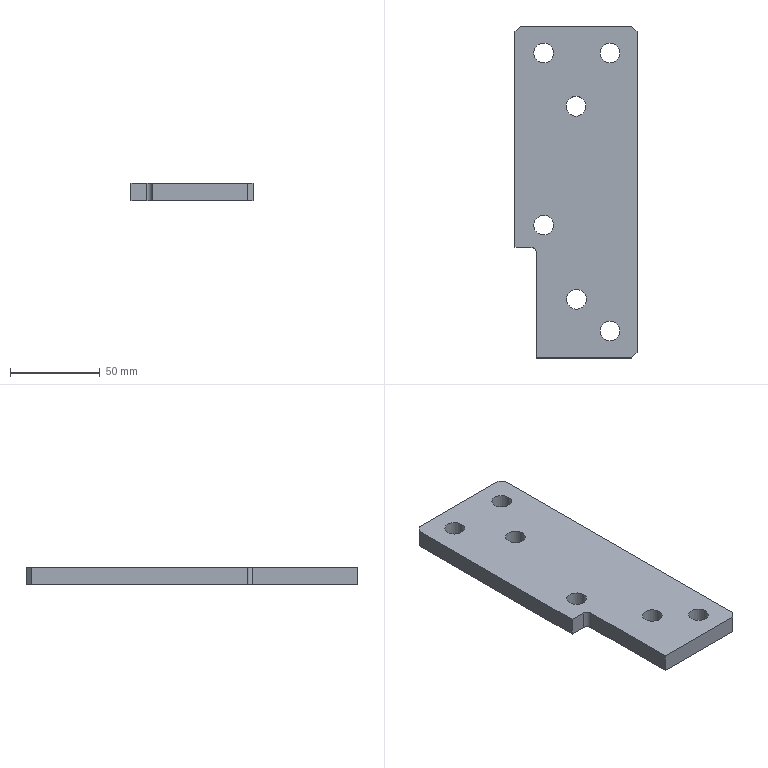Part | STEP file | 1_id182_x_t | 1 solid | 18 faces | box 68 x 185 x 10 mm | volume 112684 mm3 | plane 11 | cylinder 7 | commonest cylinder face diameters 11 x6 6 x1
STEP:
#1=CARTESIAN_POINT('',(0.,0.,0.));
#2=DIRECTION('',(0.,0.,1.));
#3=DIRECTION('',(1.,0.,0.));
#4=AXIS2_PLACEMENT_3D('',#1,#2,#3);
#5=CARTESIAN_POINT('',(251.8,221.703,100.11));
#6=VERTEX_POINT('',#5);
#7=CARTESIAN_POINT('',(246.3,221.703,100.11));
#8=DIRECTION('',(0.,0.,-1.));
#9=DIRECTION('',(1.,0.,0.));
#10=AXIS2_PLACEMENT_3D('',#7,#8,#9);
#11=CIRCLE('',#10,5.5);
#12=CARTESIAN_POINT('',(246.3,221.703,-100.11));
#13=DIRECTION('',(0.,0.,1.));
#14=DIRECTION('',(1.,0.,0.));
#15=AXIS2_PLACEMENT_3D('',#12,#13,#14);
#16=CYLINDRICAL_SURFACE('',#15,5.5);
#17=CARTESIAN_POINT('',(6.283,200.22));
#18=DIRECTION('',(-1.,0.));
#19=VECTOR('',#18,1.);
#20=LINE('',#17,#19);
#21=(GEOMETRIC_REPRESENTATION_CONTEXT(2)PARAMETRIC_REPRESENTATION_CONTEXT()REPRESENTATION_CONTEXT('',''));
#22=DEFINITIONAL_REPRESENTATION('',(#20),#21);
#23=PCURVE('',#16,#22);
#24=CARTESIAN_POINT('',(296.763,161.703,100.11));
#25=DIRECTION('',(0.,0.,1.));
#26=DIRECTION('',(1.,0.,0.));
#27=AXIS2_PLACEMENT_3D('',#24,#25,#26);
#28=PLANE('',#27);
#29=CARTESIAN_POINT('',(-44.962,60.));
#30=CARTESIAN_POINT('',(-44.962,50.474));
#31=CARTESIAN_POINT('',(-53.212,55.237));
#32=CARTESIAN_POINT('',(-61.462,60.));
#33=CARTESIAN_POINT('',(-53.212,64.763));
#34=CARTESIAN_POINT('',(-44.962,69.526));
#35=CARTESIAN_POINT('',(-44.962,60.));
#36=(BOUNDED_CURVE()B_SPLINE_CURVE(2,(#29,#30,#31,#32,#33,#34,#35),.UNSPECIFIED.,.T.,.F.)B_SPLINE_CURVE_WITH_KNOTS((1,2,2,2,2,1),(-2.094,0.,2.094,4.189,6.283,8.378),.UNSPECIFIED.)CURVE()GEOMETRIC_REPRESENTATION_ITEM()RATIONAL_B_SPLINE_CURVE((1.,0.5,1.,0.5,1.,0.5,1.))REPRESENTATION_ITEM(''));
#37=(GEOMETRIC_REPRESENTATION_CONTEXT(2)PARAMETRIC_REPRESENTATION_CONTEXT()REPRESENTATION_CONTEXT('',''));
#38=DEFINITIONAL_REPRESENTATION('',(#36),#37);
#39=PCURVE('',#28,#38);
#40=SURFACE_CURVE('',#11,(#23,#39),.PCURVE_S1.);
#41=EDGE_CURVE('',#6,#6,#40,.T.);
#42=ORIENTED_EDGE('',*,*,#41,.T.);
#43=CARTESIAN_POINT('',(251.8,221.703,90.11));
#44=VERTEX_POINT('',#43);
#45=CARTESIAN_POINT('',(251.8,221.703,90.11));
#46=CARTESIAN_POINT('',(251.8,221.703,100.11));
#47=B_SPLINE_CURVE_WITH_KNOTS('',1,(#45,#46),.UNSPECIFIED.,.F.,.F.,(2,2),(190.22,200.22),.PIECEWISE_BEZIER_KNOTS.);
#48=CARTESIAN_POINT('',(0.,0.));
#49=DIRECTION('',(0.,1.));
#50=VECTOR('',#49,1.);
#51=LINE('',#48,#50);
#52=(GEOMETRIC_REPRESENTATION_CONTEXT(2)PARAMETRIC_REPRESENTATION_CONTEXT()REPRESENTATION_CONTEXT('',''));
#53=DEFINITIONAL_REPRESENTATION('',(#51),#52);
#54=PCURVE('',#16,#53);
#55=CARTESIAN_POINT('',(6.283,0.));
#56=DIRECTION('',(0.,1.));
#57=VECTOR('',#56,1.);
#58=LINE('',#55,#57);
#59=(GEOMETRIC_REPRESENTATION_CONTEXT(2)PARAMETRIC_REPRESENTATION_CONTEXT()REPRESENTATION_CONTEXT('',''));
#60=DEFINITIONAL_REPRESENTATION('',(#58),#59);
#61=PCURVE('',#16,#60);
#62=SEAM_CURVE('',#47,(#54,#61),.PCURVE_S1.);
#63=EDGE_CURVE('',#44,#6,#62,.T.);
#64=ORIENTED_EDGE('',*,*,#63,.F.);
#65=CARTESIAN_POINT('',(246.3,221.703,90.11));
#66=DIRECTION('',(0.,0.,-1.));
#67=DIRECTION('',(1.,0.,0.));
#68=AXIS2_PLACEMENT_3D('',#65,#66,#67);
#69=CIRCLE('',#68,5.5);
#70=CARTESIAN_POINT('',(6.283,190.22));
#71=DIRECTION('',(-1.,0.));
#72=VECTOR('',#71,1.);
#73=LINE('',#70,#72);
#74=(GEOMETRIC_REPRESENTATION_CONTEXT(2)PARAMETRIC_REPRESENTATION_CONTEXT()REPRESENTATION_CONTEXT('',''));
#75=DEFINITIONAL_REPRESENTATION('',(#73),#74);
#76=PCURVE('',#16,#75);
#77=CARTESIAN_POINT('',(296.763,161.703,90.11));
#78=DIRECTION('',(0.,0.,1.));
#79=DIRECTION('',(1.,0.,0.));
#80=AXIS2_PLACEMENT_3D('',#77,#78,#79);
#81=PLANE('',#80);
#82=CARTESIAN_POINT('',(-44.962,60.));
#83=CARTESIAN_POINT('',(-44.962,50.474));
#84=CARTESIAN_POINT('',(-53.212,55.237));
#85=CARTESIAN_POINT('',(-61.462,60.));
#86=CARTESIAN_POINT('',(-53.212,64.763));
#87=CARTESIAN_POINT('',(-44.962,69.526));
#88=CARTESIAN_POINT('',(-44.962,60.));
#89=(BOUNDED_CURVE()B_SPLINE_CURVE(2,(#82,#83,#84,#85,#86,#87,#88),.UNSPECIFIED.,.T.,.F.)B_SPLINE_CURVE_WITH_KNOTS((1,2,2,2,2,1),(-2.094,0.,2.094,4.189,6.283,8.378),.UNSPECIFIED.)CURVE()GEOMETRIC_REPRESENTATION_ITEM()RATIONAL_B_SPLINE_CURVE((1.,0.5,1.,0.5,1.,0.5,1.))REPRESENTATION_ITEM(''));
#90=(GEOMETRIC_REPRESENTATION_CONTEXT(2)PARAMETRIC_REPRESENTATION_CONTEXT()REPRESENTATION_CONTEXT('',''));
#91=DEFINITIONAL_REPRESENTATION('',(#89),#90);
#92=PCURVE('',#81,#91);
#93=SURFACE_CURVE('',#69,(#76,#92),.PCURVE_S1.);
#94=EDGE_CURVE('',#44,#44,#93,.T.);
#95=ORIENTED_EDGE('',*,*,#94,.F.);
#96=ORIENTED_EDGE('',*,*,#63,.T.);
#97=EDGE_LOOP('',(#42,#64,#95,#96));
#98=FACE_BOUND('',#97,.F.);
#99=ADVANCED_FACE('',(#98),#16,.F.);
#100=CARTESIAN_POINT('',(295.3,332.703,90.11));
#101=VERTEX_POINT('',#100);
#102=CARTESIAN_POINT('',(295.3,332.703,100.11));
#103=VERTEX_POINT('',#102);
#104=CARTESIAN_POINT('',(295.3,332.703,90.11));
#105=DIRECTION('',(0.,0.,1.));
#106=VECTOR('',#105,1.);
#107=LINE('',#104,#106);
#108=CARTESIAN_POINT('',(373.531,254.472,100.11));
#109=DIRECTION('',(-0.7071,-0.7071,0.));
#110=DIRECTION('',(0.7071,-0.7071,0.));
#111=AXIS2_PLACEMENT_3D('',#108,#109,#110);
#112=PLANE('',#111);
#113=CARTESIAN_POINT('',(-110.636,-10.));
#114=DIRECTION('',(0.,1.));
#115=VECTOR('',#114,1.);
#116=LINE('',#113,#115);
#117=(GEOMETRIC_REPRESENTATION_CONTEXT(2)PARAMETRIC_REPRESENTATION_CONTEXT()REPRESENTATION_CONTEXT('',''));
#118=DEFINITIONAL_REPRESENTATION('',(#116),#117);
#119=PCURVE('',#112,#118);
#120=CARTESIAN_POINT('',(296.763,332.703,100.11));
#121=DIRECTION('',(0.,-1.,0.));
#122=DIRECTION('',(0.,0.,1.));
#123=AXIS2_PLACEMENT_3D('',#120,#121,#122);
#124=PLANE('',#123);
#125=CARTESIAN_POINT('',(-10.,1.462));
#126=DIRECTION('',(1.,0.));
#127=VECTOR('',#126,1.);
#128=LINE('',#125,#127);
#129=(GEOMETRIC_REPRESENTATION_CONTEXT(2)PARAMETRIC_REPRESENTATION_CONTEXT()REPRESENTATION_CONTEXT('',''));
#130=DEFINITIONAL_REPRESENTATION('',(#128),#129);
#131=PCURVE('',#124,#130);
#132=SURFACE_CURVE('',#107,(#119,#131),.PCURVE_S1.);
#133=EDGE_CURVE('',#101,#103,#132,.T.);
#134=ORIENTED_EDGE('',*,*,#133,.T.);
#135=CARTESIAN_POINT('',(298.3,329.703,100.11));
#136=VERTEX_POINT('',#135);
#137=CARTESIAN_POINT('',(298.3,329.703,100.11));
#138=DIRECTION('',(-0.7071,0.7071,0.));
#139=VECTOR('',#138,1.);
#140=LINE('',#137,#139);
#141=CARTESIAN_POINT('',(-106.393,0.));
#142=DIRECTION('',(-1.,0.));
#143=VECTOR('',#142,1.);
#144=LINE('',#141,#143);
#145=(GEOMETRIC_REPRESENTATION_CONTEXT(2)PARAMETRIC_REPRESENTATION_CONTEXT()REPRESENTATION_CONTEXT('',''));
#146=DEFINITIONAL_REPRESENTATION('',(#144),#145);
#147=PCURVE('',#112,#146);
#148=CARTESIAN_POINT('',(1.538,168.));
#149=DIRECTION('',(-0.7071,0.7071));
#150=VECTOR('',#149,1.);
#151=LINE('',#148,#150);
#152=(GEOMETRIC_REPRESENTATION_CONTEXT(2)PARAMETRIC_REPRESENTATION_CONTEXT()REPRESENTATION_CONTEXT('',''));
#153=DEFINITIONAL_REPRESENTATION('',(#151),#152);
#154=PCURVE('',#28,#153);
#155=SURFACE_CURVE('',#140,(#147,#154),.PCURVE_S1.);
#156=EDGE_CURVE('',#136,#103,#155,.T.);
#157=ORIENTED_EDGE('',*,*,#156,.F.);
#158=CARTESIAN_POINT('',(298.3,329.703,90.11));
#159=VERTEX_POINT('',#158);
#160=CARTESIAN_POINT('',(298.3,329.703,90.11));
#161=DIRECTION('',(0.,0.,1.));
#162=VECTOR('',#161,1.);
#163=LINE('',#160,#162);
#164=CARTESIAN_POINT('',(-106.393,-10.));
#165=DIRECTION('',(0.,1.));
#166=VECTOR('',#165,1.);
#167=LINE('',#164,#166);
#168=(GEOMETRIC_REPRESENTATION_CONTEXT(2)PARAMETRIC_REPRESENTATION_CONTEXT()REPRESENTATION_CONTEXT('',''));
#169=DEFINITIONAL_REPRESENTATION('',(#167),#168);
#170=PCURVE('',#112,#169);
#171=CARTESIAN_POINT('',(298.3,316.703,100.11));
#172=DIRECTION('',(-1.,0.,0.));
#173=DIRECTION('',(0.,-1.,0.));
#174=AXIS2_PLACEMENT_3D('',#171,#172,#173);
#175=PLANE('',#174);
#176=CARTESIAN_POINT('',(-13.,-10.));
#177=DIRECTION('',(0.,1.));
#178=VECTOR('',#177,1.);
#179=LINE('',#176,#178);
#180=(GEOMETRIC_REPRESENTATION_CONTEXT(2)PARAMETRIC_REPRESENTATION_CONTEXT()REPRESENTATION_CONTEXT('',''));
#181=DEFINITIONAL_REPRESENTATION('',(#179),#180);
#182=PCURVE('',#175,#181);
#183=SURFACE_CURVE('',#163,(#170,#182),.PCURVE_S1.);
#184=EDGE_CURVE('',#159,#136,#183,.T.);
#185=ORIENTED_EDGE('',*,*,#184,.F.);
#186=CARTESIAN_POINT('',(295.3,332.703,90.11));
#187=DIRECTION('',(0.7071,-0.7071,0.));
#188=VECTOR('',#187,1.);
#189=LINE('',#186,#188);
#190=CARTESIAN_POINT('',(-110.636,-10.));
#191=DIRECTION('',(1.,0.));
#192=VECTOR('',#191,1.);
#193=LINE('',#190,#192);
#194=(GEOMETRIC_REPRESENTATION_CONTEXT(2)PARAMETRIC_REPRESENTATION_CONTEXT()REPRESENTATION_CONTEXT('',''));
#195=DEFINITIONAL_REPRESENTATION('',(#193),#194);
#196=PCURVE('',#112,#195);
#197=CARTESIAN_POINT('',(-1.462,171.));
#198=DIRECTION('',(0.7071,-0.7071));
#199=VECTOR('',#198,1.);
#200=LINE('',#197,#199);
#201=(GEOMETRIC_REPRESENTATION_CONTEXT(2)PARAMETRIC_REPRESENTATION_CONTEXT()REPRESENTATION_CONTEXT('',''));
#202=DEFINITIONAL_REPRESENTATION('',(#200),#201);
#203=PCURVE('',#81,#202);
#204=SURFACE_CURVE('',#189,(#196,#203),.PCURVE_S1.);
#205=EDGE_CURVE('',#101,#159,#204,.T.);
#206=ORIENTED_EDGE('',*,*,#205,.F.);
#207=EDGE_LOOP('',(#134,#157,#185,#206));
#208=FACE_BOUND('',#207,.T.);
#209=ADVANCED_FACE('',(#208),#112,.F.);
#210=CARTESIAN_POINT('',(233.3,332.703,90.11));
#211=VERTEX_POINT('',#210);
#212=CARTESIAN_POINT('',(233.3,332.703,100.11));
#213=VERTEX_POINT('',#212);
#214=CARTESIAN_POINT('',(233.3,332.703,90.11));
#215=DIRECTION('',(0.,0.,1.));
#216=VECTOR('',#215,1.);
#217=LINE('',#214,#216);
#218=CARTESIAN_POINT('',(-10.,63.462));
#219=DIRECTION('',(1.,0.));
#220=VECTOR('',#219,1.);
#221=LINE('',#218,#220);
#222=(GEOMETRIC_REPRESENTATION_CONTEXT(2)PARAMETRIC_REPRESENTATION_CONTEXT()REPRESENTATION_CONTEXT('',''));
#223=DEFINITIONAL_REPRESENTATION('',(#221),#222);
#224=PCURVE('',#124,#223);
#225=CARTESIAN_POINT('',(187.531,286.935,100.11));
#226=DIRECTION('',(0.7071,-0.7071,0.));
#227=DIRECTION('',(0.7071,0.7071,0.));
#228=AXIS2_PLACEMENT_3D('',#225,#226,#227);
#229=PLANE('',#228);
#230=CARTESIAN_POINT('',(64.727,-10.));
#231=DIRECTION('',(0.,1.));
#232=VECTOR('',#231,1.);
#233=LINE('',#230,#232);
#234=(GEOMETRIC_REPRESENTATION_CONTEXT(2)PARAMETRIC_REPRESENTATION_CONTEXT()REPRESENTATION_CONTEXT('',''));
#235=DEFINITIONAL_REPRESENTATION('',(#233),#234);
#236=PCURVE('',#229,#235);
#237=SURFACE_CURVE('',#217,(#224,#236),.PCURVE_S1.);
#238=EDGE_CURVE('',#211,#213,#237,.T.);
#239=ORIENTED_EDGE('',*,*,#238,.T.);
#240=CARTESIAN_POINT('',(233.3,332.703,100.11));
#241=DIRECTION('',(1.,0.,0.));
#242=VECTOR('',#241,1.);
#243=LINE('',#240,#242);
#244=CARTESIAN_POINT('',(0.,63.462));
#245=DIRECTION('',(0.,-1.));
#246=VECTOR('',#245,1.);
#247=LINE('',#244,#246);
#248=(GEOMETRIC_REPRESENTATION_CONTEXT(2)PARAMETRIC_REPRESENTATION_CONTEXT()REPRESENTATION_CONTEXT('',''));
#249=DEFINITIONAL_REPRESENTATION('',(#247),#248);
#250=PCURVE('',#124,#249);
#251=CARTESIAN_POINT('',(-63.462,171.));
#252=DIRECTION('',(1.,0.));
#253=VECTOR('',#252,1.);
#254=LINE('',#251,#253);
#255=(GEOMETRIC_REPRESENTATION_CONTEXT(2)PARAMETRIC_REPRESENTATION_CONTEXT()REPRESENTATION_CONTEXT('',''));
#256=DEFINITIONAL_REPRESENTATION('',(#254),#255);
#257=PCURVE('',#28,#256);
#258=SURFACE_CURVE('',#243,(#250,#257),.PCURVE_S1.);
#259=EDGE_CURVE('',#213,#103,#258,.T.);
#260=ORIENTED_EDGE('',*,*,#259,.T.);
#261=ORIENTED_EDGE('',*,*,#133,.F.);
#262=CARTESIAN_POINT('',(233.3,332.703,90.11));
#263=DIRECTION('',(1.,0.,0.));
#264=VECTOR('',#263,1.);
#265=LINE('',#262,#264);
#266=CARTESIAN_POINT('',(-10.,63.462));
#267=DIRECTION('',(0.,-1.));
#268=VECTOR('',#267,1.);
#269=LINE('',#266,#268);
#270=(GEOMETRIC_REPRESENTATION_CONTEXT(2)PARAMETRIC_REPRESENTATION_CONTEXT()REPRESENTATION_CONTEXT('',''));
#271=DEFINITIONAL_REPRESENTATION('',(#269),#270);
#272=PCURVE('',#124,#271);
#273=CARTESIAN_POINT('',(-63.462,171.));
#274=DIRECTION('',(1.,0.));
#275=VECTOR('',#274,1.);
#276=LINE('',#273,#275);
#277=(GEOMETRIC_REPRESENTATION_CONTEXT(2)PARAMETRIC_REPRESENTATION_CONTEXT()REPRESENTATION_CONTEXT('',''));
#278=DEFINITIONAL_REPRESENTATION('',(#276),#277);
#279=PCURVE('',#81,#278);
#280=SURFACE_CURVE('',#265,(#272,#279),.PCURVE_S1.);
#281=EDGE_CURVE('',#211,#101,#280,.T.);
#282=ORIENTED_EDGE('',*,*,#281,.F.);
#283=EDGE_LOOP('',(#239,#260,#261,#282));
#284=FACE_BOUND('',#283,.T.);
#285=ADVANCED_FACE('',(#284),#124,.F.);
#286=CARTESIAN_POINT('',(230.3,329.703,90.11));
#287=VERTEX_POINT('',#286);
#288=CARTESIAN_POINT('',(230.3,329.703,100.11));
#289=VERTEX_POINT('',#288);
#290=CARTESIAN_POINT('',(230.3,329.703,90.11));
#291=DIRECTION('',(0.,0.,1.));
#292=VECTOR('',#291,1.);
#293=LINE('',#290,#292);
#294=CARTESIAN_POINT('',(60.484,-10.));
#295=DIRECTION('',(0.,1.));
#296=VECTOR('',#295,1.);
#297=LINE('',#294,#296);
#298=(GEOMETRIC_REPRESENTATION_CONTEXT(2)PARAMETRIC_REPRESENTATION_CONTEXT()REPRESENTATION_CONTEXT('',''));
#299=DEFINITIONAL_REPRESENTATION('',(#297),#298);
#300=PCURVE('',#229,#299);
#301=CARTESIAN_POINT('',(230.3,316.703,100.11));
#302=DIRECTION('',(1.,0.,0.));
#303=DIRECTION('',(0.,1.,0.));
#304=AXIS2_PLACEMENT_3D('',#301,#302,#303);
#305=PLANE('',#304);
#306=CARTESIAN_POINT('',(13.,-10.));
#307=DIRECTION('',(0.,1.));
#308=VECTOR('',#307,1.);
#309=LINE('',#306,#308);
#310=(GEOMETRIC_REPRESENTATION_CONTEXT(2)PARAMETRIC_REPRESENTATION_CONTEXT()REPRESENTATION_CONTEXT('',''));
#311=DEFINITIONAL_REPRESENTATION('',(#309),#310);
#312=PCURVE('',#305,#311);
#313=SURFACE_CURVE('',#293,(#300,#312),.PCURVE_S1.);
#314=EDGE_CURVE('',#287,#289,#313,.T.);
#315=ORIENTED_EDGE('',*,*,#314,.T.);
#316=CARTESIAN_POINT('',(233.3,332.703,100.11));
#317=DIRECTION('',(-0.7071,-0.7071,0.));
#318=VECTOR('',#317,1.);
#319=LINE('',#316,#318);
#320=CARTESIAN_POINT('',(64.727,0.));
#321=DIRECTION('',(-1.,0.));
#322=VECTOR('',#321,1.);
#323=LINE('',#320,#322);
#324=(GEOMETRIC_REPRESENTATION_CONTEXT(2)PARAMETRIC_REPRESENTATION_CONTEXT()REPRESENTATION_CONTEXT('',''));
#325=DEFINITIONAL_REPRESENTATION('',(#323),#324);
#326=PCURVE('',#229,#325);
#327=CARTESIAN_POINT('',(-63.462,171.));
#328=DIRECTION('',(-0.7071,-0.7071));
#329=VECTOR('',#328,1.);
#330=LINE('',#327,#329);
#331=(GEOMETRIC_REPRESENTATION_CONTEXT(2)PARAMETRIC_REPRESENTATION_CONTEXT()REPRESENTATION_CONTEXT('',''));
#332=DEFINITIONAL_REPRESENTATION('',(#330),#331);
#333=PCURVE('',#28,#332);
#334=SURFACE_CURVE('',#319,(#326,#333),.PCURVE_S1.);
#335=EDGE_CURVE('',#213,#289,#334,.T.);
#336=ORIENTED_EDGE('',*,*,#335,.F.);
#337=ORIENTED_EDGE('',*,*,#238,.F.);
#338=CARTESIAN_POINT('',(230.3,329.703,90.11));
#339=DIRECTION('',(0.7071,0.7071,0.));
#340=VECTOR('',#339,1.);
#341=LINE('',#338,#340);
#342=CARTESIAN_POINT('',(60.484,-10.));
#343=DIRECTION('',(1.,0.));
#344=VECTOR('',#343,1.);
#345=LINE('',#342,#344);
#346=(GEOMETRIC_REPRESENTATION_CONTEXT(2)PARAMETRIC_REPRESENTATION_CONTEXT()REPRESENTATION_CONTEXT('',''));
#347=DEFINITIONAL_REPRESENTATION('',(#345),#346);
#348=PCURVE('',#229,#347);
#349=CARTESIAN_POINT('',(-66.463,168.));
#350=DIRECTION('',(0.7071,0.7071));
#351=VECTOR('',#350,1.);
#352=LINE('',#349,#351);
#353=(GEOMETRIC_REPRESENTATION_CONTEXT(2)PARAMETRIC_REPRESENTATION_CONTEXT()REPRESENTATION_CONTEXT('',''));
#354=DEFINITIONAL_REPRESENTATION('',(#352),#353);
#355=PCURVE('',#81,#354);
#356=SURFACE_CURVE('',#341,(#348,#355),.PCURVE_S1.);
#357=EDGE_CURVE('',#287,#211,#356,.T.);
#358=ORIENTED_EDGE('',*,*,#357,.F.);
#359=EDGE_LOOP('',(#315,#336,#337,#358));
#360=FACE_BOUND('',#359,.T.);
#361=ADVANCED_FACE('',(#360),#229,.F.);
#362=CARTESIAN_POINT('',(230.3,209.297,100.11));
#363=VERTEX_POINT('',#362);
#364=CARTESIAN_POINT('',(230.3,209.297,100.11));
#365=DIRECTION('',(0.,1.,0.));
#366=VECTOR('',#365,1.);
#367=LINE('',#364,#366);
#368=CARTESIAN_POINT('',(-107.407,0.));
#369=DIRECTION('',(1.,0.));
#370=VECTOR('',#369,1.);
#371=LINE('',#368,#370);
#372=(GEOMETRIC_REPRESENTATION_CONTEXT(2)PARAMETRIC_REPRESENTATION_CONTEXT()REPRESENTATION_CONTEXT('',''));
#373=DEFINITIONAL_REPRESENTATION('',(#371),#372);
#374=PCURVE('',#305,#373);
#375=CARTESIAN_POINT('',(-66.463,47.593));
#376=DIRECTION('',(0.,1.));
#377=VECTOR('',#376,1.);
#378=LINE('',#375,#377);
#379=(GEOMETRIC_REPRESENTATION_CONTEXT(2)PARAMETRIC_REPRESENTATION_CONTEXT()REPRESENTATION_CONTEXT('',''));
#380=DEFINITIONAL_REPRESENTATION('',(#378),#379);
#381=PCURVE('',#28,#380);
#382=SURFACE_CURVE('',#367,(#374,#381),.PCURVE_S1.);
#383=EDGE_CURVE('',#363,#289,#382,.T.);
#384=ORIENTED_EDGE('',*,*,#383,.T.);
#385=ORIENTED_EDGE('',*,*,#314,.F.);
#386=CARTESIAN_POINT('',(230.3,209.297,90.11));
#387=VERTEX_POINT('',#386);
#388=CARTESIAN_POINT('',(230.3,209.297,90.11));
#389=DIRECTION('',(0.,1.,0.));
#390=VECTOR('',#389,1.);
#391=LINE('',#388,#390);
#392=CARTESIAN_POINT('',(-107.407,-10.));
#393=DIRECTION('',(1.,0.));
#394=VECTOR('',#393,1.);
#395=LINE('',#392,#394);
#396=(GEOMETRIC_REPRESENTATION_CONTEXT(2)PARAMETRIC_REPRESENTATION_CONTEXT()REPRESENTATION_CONTEXT('',''));
#397=DEFINITIONAL_REPRESENTATION('',(#395),#396);
#398=PCURVE('',#305,#397);
#399=CARTESIAN_POINT('',(-66.463,47.593));
#400=DIRECTION('',(0.,1.));
#401=VECTOR('',#400,1.);
#402=LINE('',#399,#401);
#403=(GEOMETRIC_REPRESENTATION_CONTEXT(2)PARAMETRIC_REPRESENTATION_CONTEXT()REPRESENTATION_CONTEXT('',''));
#404=DEFINITIONAL_REPRESENTATION('',(#402),#403);
#405=PCURVE('',#81,#404);
#406=SURFACE_CURVE('',#391,(#398,#405),.PCURVE_S1.);
#407=EDGE_CURVE('',#387,#287,#406,.T.);
#408=ORIENTED_EDGE('',*,*,#407,.F.);
#409=CARTESIAN_POINT('',(230.3,209.297,90.11));
#410=DIRECTION('',(0.,0.,1.));
#411=VECTOR('',#410,1.);
#412=LINE('',#409,#411);
#413=CARTESIAN_POINT('',(-107.407,-10.));
#414=DIRECTION('',(0.,1.));
#415=VECTOR('',#414,1.);
#416=LINE('',#413,#415);
#417=(GEOMETRIC_REPRESENTATION_CONTEXT(2)PARAMETRIC_REPRESENTATION_CONTEXT()REPRESENTATION_CONTEXT('',''));
#418=DEFINITIONAL_REPRESENTATION('',(#416),#417);
#419=PCURVE('',#305,#418);
#420=CARTESIAN_POINT('',(174.688,209.297,100.11));
#421=DIRECTION('',(0.,-1.,0.));
#422=DIRECTION('',(0.,0.,-1.));
#423=AXIS2_PLACEMENT_3D('',#420,#421,#422);
#424=PLANE('',#423);
#425=CARTESIAN_POINT('',(10.,55.612));
#426=DIRECTION('',(-1.,0.));
#427=VECTOR('',#426,1.);
#428=LINE('',#425,#427);
#429=(GEOMETRIC_REPRESENTATION_CONTEXT(2)PARAMETRIC_REPRESENTATION_CONTEXT()REPRESENTATION_CONTEXT('',''));
#430=DEFINITIONAL_REPRESENTATION('',(#428),#429);
#431=PCURVE('',#424,#430);
#432=SURFACE_CURVE('',#412,(#419,#431),.PCURVE_S1.);
#433=EDGE_CURVE('',#387,#363,#432,.T.);
#434=ORIENTED_EDGE('',*,*,#433,.T.);
#435=EDGE_LOOP('',(#384,#385,#408,#434));
#436=FACE_BOUND('',#435,.T.);
#437=ADVANCED_FACE('',(#436),#305,.F.);
#438=CARTESIAN_POINT('',(239.15,209.297,100.11));
#439=VERTEX_POINT('',#438);
#440=CARTESIAN_POINT('',(239.15,209.297,90.11));
#441=VERTEX_POINT('',#440);
#442=CARTESIAN_POINT('',(239.15,209.297,100.11));
#443=DIRECTION('',(0.,0.,-1.));
#444=VECTOR('',#443,1.);
#445=LINE('',#442,#444);
#446=CARTESIAN_POINT('',(0.,64.463));
#447=DIRECTION('',(1.,0.));
#448=VECTOR('',#447,1.);
#449=LINE('',#446,#448);
#450=(GEOMETRIC_REPRESENTATION_CONTEXT(2)PARAMETRIC_REPRESENTATION_CONTEXT()REPRESENTATION_CONTEXT('',''));
#451=DEFINITIONAL_REPRESENTATION('',(#449),#450);
#452=PCURVE('',#424,#451);
#453=CARTESIAN_POINT('',(239.15,206.297,100.11));
#454=DIRECTION('',(0.,0.,-1.));
#455=DIRECTION('',(-1.,0.,0.));
#456=AXIS2_PLACEMENT_3D('',#453,#454,#455);
#457=CYLINDRICAL_SURFACE('',#456,3.);
#458=CARTESIAN_POINT('',(1.571,0.));
#459=DIRECTION('',(0.,1.));
#460=VECTOR('',#459,1.);
#461=LINE('',#458,#460);
#462=(GEOMETRIC_REPRESENTATION_CONTEXT(2)PARAMETRIC_REPRESENTATION_CONTEXT()REPRESENTATION_CONTEXT('',''));
#463=DEFINITIONAL_REPRESENTATION('',(#461),#462);
#464=PCURVE('',#457,#463);
#465=SURFACE_CURVE('',#445,(#452,#464),.PCURVE_S1.);
#466=EDGE_CURVE('',#439,#441,#465,.T.);
#467=ORIENTED_EDGE('',*,*,#466,.F.);
#468=CARTESIAN_POINT('',(239.15,209.297,100.11));
#469=DIRECTION('',(-1.,0.,0.));
#470=VECTOR('',#469,1.);
#471=LINE('',#468,#470);
#472=CARTESIAN_POINT('',(0.,64.463));
#473=DIRECTION('',(0.,-1.));
#474=VECTOR('',#473,1.);
#475=LINE('',#472,#474);
#476=(GEOMETRIC_REPRESENTATION_CONTEXT(2)PARAMETRIC_REPRESENTATION_CONTEXT()REPRESENTATION_CONTEXT('',''));
#477=DEFINITIONAL_REPRESENTATION('',(#475),#476);
#478=PCURVE('',#424,#477);
#479=CARTESIAN_POINT('',(-57.612,47.593));
#480=DIRECTION('',(-1.,0.));
#481=VECTOR('',#480,1.);
#482=LINE('',#479,#481);
#483=(GEOMETRIC_REPRESENTATION_CONTEXT(2)PARAMETRIC_REPRESENTATION_CONTEXT()REPRESENTATION_CONTEXT('',''));
#484=DEFINITIONAL_REPRESENTATION('',(#482),#483);
#485=PCURVE('',#28,#484);
#486=SURFACE_CURVE('',#471,(#478,#485),.PCURVE_S1.);
#487=EDGE_CURVE('',#439,#363,#486,.T.);
#488=ORIENTED_EDGE('',*,*,#487,.T.);
#489=ORIENTED_EDGE('',*,*,#433,.F.);
#490=CARTESIAN_POINT('',(239.15,209.297,90.11));
#491=DIRECTION('',(-1.,0.,0.));
#492=VECTOR('',#491,1.);
#493=LINE('',#490,#492);
#494=CARTESIAN_POINT('',(10.,64.463));
#495=DIRECTION('',(0.,-1.));
#496=VECTOR('',#495,1.);
#497=LINE('',#494,#496);
#498=(GEOMETRIC_REPRESENTATION_CONTEXT(2)PARAMETRIC_REPRESENTATION_CONTEXT()REPRESENTATION_CONTEXT('',''));
#499=DEFINITIONAL_REPRESENTATION('',(#497),#498);
#500=PCURVE('',#424,#499);
#501=CARTESIAN_POINT('',(-57.612,47.593));
#502=DIRECTION('',(-1.,0.));
#503=VECTOR('',#502,1.);
#504=LINE('',#501,#503);
#505=(GEOMETRIC_REPRESENTATION_CONTEXT(2)PARAMETRIC_REPRESENTATION_CONTEXT()REPRESENTATION_CONTEXT('',''));
#506=DEFINITIONAL_REPRESENTATION('',(#504),#505);
#507=PCURVE('',#81,#506);
#508=SURFACE_CURVE('',#493,(#500,#507),.PCURVE_S1.);
#509=EDGE_CURVE('',#441,#387,#508,.T.);
#510=ORIENTED_EDGE('',*,*,#509,.F.);
#511=EDGE_LOOP('',(#467,#488,#489,#510));
#512=FACE_BOUND('',#511,.T.);
#513=ADVANCED_FACE('',(#512),#424,.T.);
#514=CARTESIAN_POINT('',(242.15,206.297,90.11));
#515=VERTEX_POINT('',#514);
#516=CARTESIAN_POINT('',(239.15,206.297,90.11));
#517=DIRECTION('',(0.,0.,1.));
#518=DIRECTION('',(1.,0.,0.));
#519=AXIS2_PLACEMENT_3D('',#516,#517,#518);
#520=CIRCLE('',#519,3.);
#521=CARTESIAN_POINT('',(3.142,10.));
#522=DIRECTION('',(-1.,0.));
#523=VECTOR('',#522,1.);
#524=LINE('',#521,#523);
#525=(GEOMETRIC_REPRESENTATION_CONTEXT(2)PARAMETRIC_REPRESENTATION_CONTEXT()REPRESENTATION_CONTEXT('',''));
#526=DEFINITIONAL_REPRESENTATION('',(#524),#525);
#527=PCURVE('',#457,#526);
#528=CARTESIAN_POINT('',(-57.612,44.593));
#529=DIRECTION('',(1.,0.));
#530=AXIS2_PLACEMENT_2D('',#528,#529);
#531=CIRCLE('',#530,3.);
#532=(GEOMETRIC_REPRESENTATION_CONTEXT(2)PARAMETRIC_REPRESENTATION_CONTEXT()REPRESENTATION_CONTEXT('',''));
#533=DEFINITIONAL_REPRESENTATION('',(#531),#532);
#534=PCURVE('',#81,#533);
#535=SURFACE_CURVE('',#520,(#527,#534),.PCURVE_S1.);
#536=EDGE_CURVE('',#515,#441,#535,.T.);
#537=ORIENTED_EDGE('',*,*,#536,.T.);
#538=ORIENTED_EDGE('',*,*,#466,.F.);
#539=CARTESIAN_POINT('',(242.15,206.297,100.11));
#540=VERTEX_POINT('',#539);
#541=CARTESIAN_POINT('',(239.15,206.297,100.11));
#542=DIRECTION('',(0.,0.,-1.));
#543=DIRECTION('',(0.,1.,0.));
#544=AXIS2_PLACEMENT_3D('',#541,#542,#543);
#545=CIRCLE('',#544,3.);
#546=CARTESIAN_POINT('',(1.571,0.));
#547=DIRECTION('',(1.,0.));
#548=VECTOR('',#547,1.);
#549=LINE('',#546,#548);
#550=(GEOMETRIC_REPRESENTATION_CONTEXT(2)PARAMETRIC_REPRESENTATION_CONTEXT()REPRESENTATION_CONTEXT('',''));
#551=DEFINITIONAL_REPRESENTATION('',(#549),#550);
#552=PCURVE('',#457,#551);
#553=CARTESIAN_POINT('',(-57.612,47.593));
#554=CARTESIAN_POINT('',(-52.416,47.593));
#555=CARTESIAN_POINT('',(-55.014,43.093));
#556=CARTESIAN_POINT('',(-57.612,38.593));
#557=CARTESIAN_POINT('',(-60.211,43.093));
#558=CARTESIAN_POINT('',(-62.809,47.593));
#559=CARTESIAN_POINT('',(-57.612,47.593));
#560=(BOUNDED_CURVE()B_SPLINE_CURVE(2,(#553,#554,#555,#556,#557,#558,#559),.UNSPECIFIED.,.T.,.F.)B_SPLINE_CURVE_WITH_KNOTS((1,2,2,2,2,1),(-2.094,0.,2.094,4.189,6.283,8.378),.UNSPECIFIED.)CURVE()GEOMETRIC_REPRESENTATION_ITEM()RATIONAL_B_SPLINE_CURVE((1.,0.5,1.,0.5,1.,0.5,1.))REPRESENTATION_ITEM(''));
#561=(GEOMETRIC_REPRESENTATION_CONTEXT(2)PARAMETRIC_REPRESENTATION_CONTEXT()REPRESENTATION_CONTEXT('',''));
#562=DEFINITIONAL_REPRESENTATION('',(#560),#561);
#563=PCURVE('',#28,#562);
#564=SURFACE_CURVE('',#545,(#552,#563),.PCURVE_S1.);
#565=EDGE_CURVE('',#439,#540,#564,.T.);
#566=ORIENTED_EDGE('',*,*,#565,.T.);
#567=CARTESIAN_POINT('',(242.15,206.297,90.11));
#568=DIRECTION('',(0.,0.,1.));
#569=VECTOR('',#568,1.);
#570=LINE('',#567,#569);
#571=CARTESIAN_POINT('',(3.142,10.));
#572=DIRECTION('',(0.,-1.));
#573=VECTOR('',#572,1.);
#574=LINE('',#571,#573);
#575=(GEOMETRIC_REPRESENTATION_CONTEXT(2)PARAMETRIC_REPRESENTATION_CONTEXT()REPRESENTATION_CONTEXT('',''));
#576=DEFINITIONAL_REPRESENTATION('',(#574),#575);
#577=PCURVE('',#457,#576);
#578=CARTESIAN_POINT('',(242.15,38.297,100.11));
#579=DIRECTION('',(-1.,0.,0.));
#580=DIRECTION('',(0.,1.,0.));
#581=AXIS2_PLACEMENT_3D('',#578,#579,#580);
#582=PLANE('',#581);
#583=CARTESIAN_POINT('',(168.,10.));
#584=DIRECTION('',(0.,-1.));
#585=VECTOR('',#584,1.);
#586=LINE('',#583,#585);
#587=(GEOMETRIC_REPRESENTATION_CONTEXT(2)PARAMETRIC_REPRESENTATION_CONTEXT()REPRESENTATION_CONTEXT('',''));
#588=DEFINITIONAL_REPRESENTATION('',(#586),#587);
#589=PCURVE('',#582,#588);
#590=SURFACE_CURVE('',#570,(#577,#589),.PCURVE_S1.);
#591=EDGE_CURVE('',#515,#540,#590,.T.);
#592=ORIENTED_EDGE('',*,*,#591,.F.);
#593=EDGE_LOOP('',(#537,#538,#566,#592));
#594=FACE_BOUND('',#593,.F.);
#595=ADVANCED_FACE('',(#594),#457,.F.);
#596=ORIENTED_EDGE('',*,*,#591,.F.);
#597=CARTESIAN_POINT('',(242.15,147.703,90.11));
#598=VERTEX_POINT('',#597);
#599=CARTESIAN_POINT('',(242.15,147.703,90.11));
#600=DIRECTION('',(0.,1.,0.));
#601=VECTOR('',#600,1.);
#602=LINE('',#599,#601);
#603=CARTESIAN_POINT('',(109.407,10.));
#604=DIRECTION('',(1.,0.));
#605=VECTOR('',#604,1.);
#606=LINE('',#603,#605);
#607=(GEOMETRIC_REPRESENTATION_CONTEXT(2)PARAMETRIC_REPRESENTATION_CONTEXT()REPRESENTATION_CONTEXT('',''));
#608=DEFINITIONAL_REPRESENTATION('',(#606),#607);
#609=PCURVE('',#582,#608);
#610=CARTESIAN_POINT('',(-54.612,-14.));
#611=DIRECTION('',(0.,1.));
#612=VECTOR('',#611,1.);
#613=LINE('',#610,#612);
#614=(GEOMETRIC_REPRESENTATION_CONTEXT(2)PARAMETRIC_REPRESENTATION_CONTEXT()REPRESENTATION_CONTEXT('',''));
#615=DEFINITIONAL_REPRESENTATION('',(#613),#614);
#616=PCURVE('',#81,#615);
#617=SURFACE_CURVE('',#602,(#609,#616),.PCURVE_S1.);
#618=EDGE_CURVE('',#598,#515,#617,.T.);
#619=ORIENTED_EDGE('',*,*,#618,.F.);
#620=CARTESIAN_POINT('',(242.15,147.703,100.11));
#621=VERTEX_POINT('',#620);
#622=CARTESIAN_POINT('',(242.15,147.703,100.11));
#623=DIRECTION('',(0.,0.,-1.));
#624=VECTOR('',#623,1.);
#625=LINE('',#622,#624);
#626=CARTESIAN_POINT('',(109.407,0.));
#627=DIRECTION('',(0.,1.));
#628=VECTOR('',#627,1.);
#629=LINE('',#626,#628);
#630=(GEOMETRIC_REPRESENTATION_CONTEXT(2)PARAMETRIC_REPRESENTATION_CONTEXT()REPRESENTATION_CONTEXT('',''));
#631=DEFINITIONAL_REPRESENTATION('',(#629),#630);
#632=PCURVE('',#582,#631);
#633=CARTESIAN_POINT('',(231.838,147.703,100.11));
#634=DIRECTION('',(0.,1.,0.));
#635=DIRECTION('',(0.,0.,-1.));
#636=AXIS2_PLACEMENT_3D('',#633,#634,#635);
#637=PLANE('',#636);
#638=CARTESIAN_POINT('',(0.,-10.312));
#639=DIRECTION('',(1.,0.));
#640=VECTOR('',#639,1.);
#641=LINE('',#638,#640);
#642=(GEOMETRIC_REPRESENTATION_CONTEXT(2)PARAMETRIC_REPRESENTATION_CONTEXT()REPRESENTATION_CONTEXT('',''));
#643=DEFINITIONAL_REPRESENTATION('',(#641),#642);
#644=PCURVE('',#637,#643);
#645=SURFACE_CURVE('',#625,(#632,#644),.PCURVE_S1.);
#646=EDGE_CURVE('',#621,#598,#645,.T.);
#647=ORIENTED_EDGE('',*,*,#646,.F.);
#648=CARTESIAN_POINT('',(242.15,147.703,100.11));
#649=DIRECTION('',(0.,1.,0.));
#650=VECTOR('',#649,1.);
#651=LINE('',#648,#650);
#652=CARTESIAN_POINT('',(109.407,0.));
#653=DIRECTION('',(1.,0.));
#654=VECTOR('',#653,1.);
#655=LINE('',#652,#654);
#656=(GEOMETRIC_REPRESENTATION_CONTEXT(2)PARAMETRIC_REPRESENTATION_CONTEXT()REPRESENTATION_CONTEXT('',''));
#657=DEFINITIONAL_REPRESENTATION('',(#655),#656);
#658=PCURVE('',#582,#657);
#659=CARTESIAN_POINT('',(-54.612,-14.));
#660=DIRECTION('',(0.,1.));
#661=VECTOR('',#660,1.);
#662=LINE('',#659,#661);
#663=(GEOMETRIC_REPRESENTATION_CONTEXT(2)PARAMETRIC_REPRESENTATION_CONTEXT()REPRESENTATION_CONTEXT('',''));
#664=DEFINITIONAL_REPRESENTATION('',(#662),#663);
#665=PCURVE('',#28,#664);
#666=SURFACE_CURVE('',#651,(#658,#665),.PCURVE_S1.);
#667=EDGE_CURVE('',#621,#540,#666,.T.);
#668=ORIENTED_EDGE('',*,*,#667,.T.);
#669=EDGE_LOOP('',(#596,#619,#647,#668));
#670=FACE_BOUND('',#669,.T.);
#671=ADVANCED_FACE('',(#670),#582,.T.);
#672=CARTESIAN_POINT('',(295.3,147.703,90.11));
#673=VERTEX_POINT('',#672);
#674=CARTESIAN_POINT('',(295.3,147.703,90.11));
#675=DIRECTION('',(-1.,0.,0.));
#676=VECTOR('',#675,1.);
#677=LINE('',#674,#676);
#678=CARTESIAN_POINT('',(10.,-63.462));
#679=DIRECTION('',(0.,1.));
#680=VECTOR('',#679,1.);
#681=LINE('',#678,#680);
#682=(GEOMETRIC_REPRESENTATION_CONTEXT(2)PARAMETRIC_REPRESENTATION_CONTEXT()REPRESENTATION_CONTEXT('',''));
#683=DEFINITIONAL_REPRESENTATION('',(#681),#682);
#684=PCURVE('',#637,#683);
#685=CARTESIAN_POINT('',(-1.462,-14.));
#686=DIRECTION('',(-1.,0.));
#687=VECTOR('',#686,1.);
#688=LINE('',#685,#687);
#689=(GEOMETRIC_REPRESENTATION_CONTEXT(2)PARAMETRIC_REPRESENTATION_CONTEXT()REPRESENTATION_CONTEXT('',''));
#690=DEFINITIONAL_REPRESENTATION('',(#688),#689);
#691=PCURVE('',#81,#690);
#692=SURFACE_CURVE('',#677,(#684,#691),.PCURVE_S1.);
#693=EDGE_CURVE('',#673,#598,#692,.T.);
#694=ORIENTED_EDGE('',*,*,#693,.F.);
#695=CARTESIAN_POINT('',(295.3,147.703,100.11));
#696=VERTEX_POINT('',#695);
#697=CARTESIAN_POINT('',(295.3,147.703,90.11));
#698=DIRECTION('',(0.,0.,1.));
#699=VECTOR('',#698,1.);
#700=LINE('',#697,#699);
#701=CARTESIAN_POINT('',(10.,-63.462));
#702=DIRECTION('',(-1.,0.));
#703=VECTOR('',#702,1.);
#704=LINE('',#701,#703);
#705=(GEOMETRIC_REPRESENTATION_CONTEXT(2)PARAMETRIC_REPRESENTATION_CONTEXT()REPRESENTATION_CONTEXT('',''));
#706=DEFINITIONAL_REPRESENTATION('',(#704),#705);
#707=PCURVE('',#637,#706);
#708=CARTESIAN_POINT('',(296.031,148.435,100.11));
#709=DIRECTION('',(-0.7071,0.7071,0.));
#710=DIRECTION('',(-0.7071,-0.7071,0.));
#711=AXIS2_PLACEMENT_3D('',#708,#709,#710);
#712=PLANE('',#711);
#713=CARTESIAN_POINT('',(1.034,-10.));
#714=DIRECTION('',(0.,1.));
#715=VECTOR('',#714,1.);
#716=LINE('',#713,#715);
#717=(GEOMETRIC_REPRESENTATION_CONTEXT(2)PARAMETRIC_REPRESENTATION_CONTEXT()REPRESENTATION_CONTEXT('',''));
#718=DEFINITIONAL_REPRESENTATION('',(#716),#717);
#719=PCURVE('',#712,#718);
#720=SURFACE_CURVE('',#700,(#707,#719),.PCURVE_S1.);
#721=EDGE_CURVE('',#673,#696,#720,.T.);
#722=ORIENTED_EDGE('',*,*,#721,.T.);
#723=CARTESIAN_POINT('',(295.3,147.703,100.11));
#724=DIRECTION('',(-1.,0.,0.));
#725=VECTOR('',#724,1.);
#726=LINE('',#723,#725);
#727=CARTESIAN_POINT('',(0.,-63.462));
#728=DIRECTION('',(0.,1.));
#729=VECTOR('',#728,1.);
#730=LINE('',#727,#729);
#731=(GEOMETRIC_REPRESENTATION_CONTEXT(2)PARAMETRIC_REPRESENTATION_CONTEXT()REPRESENTATION_CONTEXT('',''));
#732=DEFINITIONAL_REPRESENTATION('',(#730),#731);
#733=PCURVE('',#637,#732);
#734=CARTESIAN_POINT('',(-1.462,-14.));
#735=DIRECTION('',(-1.,0.));
#736=VECTOR('',#735,1.);
#737=LINE('',#734,#736);
#738=(GEOMETRIC_REPRESENTATION_CONTEXT(2)PARAMETRIC_REPRESENTATION_CONTEXT()REPRESENTATION_CONTEXT('',''));
#739=DEFINITIONAL_REPRESENTATION('',(#737),#738);
#740=PCURVE('',#28,#739);
#741=SURFACE_CURVE('',#726,(#733,#740),.PCURVE_S1.);
#742=EDGE_CURVE('',#696,#621,#741,.T.);
#743=ORIENTED_EDGE('',*,*,#742,.T.);
#744=ORIENTED_EDGE('',*,*,#646,.T.);
#745=EDGE_LOOP('',(#694,#722,#743,#744));
#746=FACE_BOUND('',#745,.T.);
#747=ADVANCED_FACE('',(#746),#637,.F.);
#748=CARTESIAN_POINT('',(298.3,150.703,90.11));
#749=VERTEX_POINT('',#748);
#750=CARTESIAN_POINT('',(298.3,150.703,100.11));
#751=VERTEX_POINT('',#750);
#752=CARTESIAN_POINT('',(298.3,150.703,90.11));
#753=DIRECTION('',(0.,0.,1.));
#754=VECTOR('',#753,1.);
#755=LINE('',#752,#754);
#756=CARTESIAN_POINT('',(-3.208,-10.));
#757=DIRECTION('',(0.,1.));
#758=VECTOR('',#757,1.);
#759=LINE('',#756,#758);
#760=(GEOMETRIC_REPRESENTATION_CONTEXT(2)PARAMETRIC_REPRESENTATION_CONTEXT()REPRESENTATION_CONTEXT('',''));
#761=DEFINITIONAL_REPRESENTATION('',(#759),#760);
#762=PCURVE('',#712,#761);
#763=CARTESIAN_POINT('',(166.,-10.));
#764=DIRECTION('',(0.,1.));
#765=VECTOR('',#764,1.);
#766=LINE('',#763,#765);
#767=(GEOMETRIC_REPRESENTATION_CONTEXT(2)PARAMETRIC_REPRESENTATION_CONTEXT()REPRESENTATION_CONTEXT('',''));
#768=DEFINITIONAL_REPRESENTATION('',(#766),#767);
#769=PCURVE('',#175,#768);
#770=SURFACE_CURVE('',#755,(#762,#769),.PCURVE_S1.);
#771=EDGE_CURVE('',#749,#751,#770,.T.);
#772=ORIENTED_EDGE('',*,*,#771,.T.);
#773=CARTESIAN_POINT('',(295.3,147.703,100.11));
#774=DIRECTION('',(0.7071,0.7071,0.));
#775=VECTOR('',#774,1.);
#776=LINE('',#773,#775);
#777=CARTESIAN_POINT('',(1.034,0.));
#778=DIRECTION('',(-1.,0.));
#779=VECTOR('',#778,1.);
#780=LINE('',#777,#779);
#781=(GEOMETRIC_REPRESENTATION_CONTEXT(2)PARAMETRIC_REPRESENTATION_CONTEXT()REPRESENTATION_CONTEXT('',''));
#782=DEFINITIONAL_REPRESENTATION('',(#780),#781);
#783=PCURVE('',#712,#782);
#784=CARTESIAN_POINT('',(-1.462,-14.));
#785=DIRECTION('',(0.7071,0.7071));
#786=VECTOR('',#785,1.);
#787=LINE('',#784,#786);
#788=(GEOMETRIC_REPRESENTATION_CONTEXT(2)PARAMETRIC_REPRESENTATION_CONTEXT()REPRESENTATION_CONTEXT('',''));
#789=DEFINITIONAL_REPRESENTATION('',(#787),#788);
#790=PCURVE('',#28,#789);
#791=SURFACE_CURVE('',#776,(#783,#790),.PCURVE_S1.);
#792=EDGE_CURVE('',#696,#751,#791,.T.);
#793=ORIENTED_EDGE('',*,*,#792,.F.);
#794=ORIENTED_EDGE('',*,*,#721,.F.);
#795=CARTESIAN_POINT('',(298.3,150.703,90.11));
#796=DIRECTION('',(-0.7071,-0.7071,0.));
#797=VECTOR('',#796,1.);
#798=LINE('',#795,#797);
#799=CARTESIAN_POINT('',(-3.208,-10.));
#800=DIRECTION('',(1.,0.));
#801=VECTOR('',#800,1.);
#802=LINE('',#799,#801);
#803=(GEOMETRIC_REPRESENTATION_CONTEXT(2)PARAMETRIC_REPRESENTATION_CONTEXT()REPRESENTATION_CONTEXT('',''));
#804=DEFINITIONAL_REPRESENTATION('',(#802),#803);
#805=PCURVE('',#712,#804);
#806=CARTESIAN_POINT('',(1.538,-11.));
#807=DIRECTION('',(-0.7071,-0.7071));
#808=VECTOR('',#807,1.);
#809=LINE('',#806,#808);
#810=(GEOMETRIC_REPRESENTATION_CONTEXT(2)PARAMETRIC_REPRESENTATION_CONTEXT()REPRESENTATION_CONTEXT('',''));
#811=DEFINITIONAL_REPRESENTATION('',(#809),#810);
#812=PCURVE('',#81,#811);
#813=SURFACE_CURVE('',#798,(#805,#812),.PCURVE_S1.);
#814=EDGE_CURVE('',#749,#673,#813,.T.);
#815=ORIENTED_EDGE('',*,*,#814,.F.);
#816=EDGE_LOOP('',(#772,#793,#794,#815));
#817=FACE_BOUND('',#816,.T.);
#818=ADVANCED_FACE('',(#817),#712,.F.);
#819=ORIENTED_EDGE('',*,*,#184,.T.);
#820=CARTESIAN_POINT('',(298.3,329.703,100.11));
#821=DIRECTION('',(0.,-1.,0.));
#822=VECTOR('',#821,1.);
#823=LINE('',#820,#822);
#824=CARTESIAN_POINT('',(-13.,0.));
#825=DIRECTION('',(1.,0.));
#826=VECTOR('',#825,1.);
#827=LINE('',#824,#826);
#828=(GEOMETRIC_REPRESENTATION_CONTEXT(2)PARAMETRIC_REPRESENTATION_CONTEXT()REPRESENTATION_CONTEXT('',''));
#829=DEFINITIONAL_REPRESENTATION('',(#827),#828);
#830=PCURVE('',#175,#829);
#831=CARTESIAN_POINT('',(1.538,168.));
#832=DIRECTION('',(0.,-1.));
#833=VECTOR('',#832,1.);
#834=LINE('',#831,#833);
#835=(GEOMETRIC_REPRESENTATION_CONTEXT(2)PARAMETRIC_REPRESENTATION_CONTEXT()REPRESENTATION_CONTEXT('',''));
#836=DEFINITIONAL_REPRESENTATION('',(#834),#835);
#837=PCURVE('',#28,#836);
#838=SURFACE_CURVE('',#823,(#830,#837),.PCURVE_S1.);
#839=EDGE_CURVE('',#136,#751,#838,.T.);
#840=ORIENTED_EDGE('',*,*,#839,.T.);
#841=ORIENTED_EDGE('',*,*,#771,.F.);
#842=CARTESIAN_POINT('',(298.3,329.703,90.11));
#843=DIRECTION('',(0.,-1.,0.));
#844=VECTOR('',#843,1.);
#845=LINE('',#842,#844);
#846=CARTESIAN_POINT('',(-13.,-10.));
#847=DIRECTION('',(1.,0.));
#848=VECTOR('',#847,1.);
#849=LINE('',#846,#848);
#850=(GEOMETRIC_REPRESENTATION_CONTEXT(2)PARAMETRIC_REPRESENTATION_CONTEXT()REPRESENTATION_CONTEXT('',''));
#851=DEFINITIONAL_REPRESENTATION('',(#849),#850);
#852=PCURVE('',#175,#851);
#853=CARTESIAN_POINT('',(1.538,168.));
#854=DIRECTION('',(0.,-1.));
#855=VECTOR('',#854,1.);
#856=LINE('',#853,#855);
#857=(GEOMETRIC_REPRESENTATION_CONTEXT(2)PARAMETRIC_REPRESENTATION_CONTEXT()REPRESENTATION_CONTEXT('',''));
#858=DEFINITIONAL_REPRESENTATION('',(#856),#857);
#859=PCURVE('',#81,#858);
#860=SURFACE_CURVE('',#845,(#852,#859),.PCURVE_S1.);
#861=EDGE_CURVE('',#159,#749,#860,.T.);
#862=ORIENTED_EDGE('',*,*,#861,.F.);
#863=EDGE_LOOP('',(#819,#840,#841,#862));
#864=FACE_BOUND('',#863,.T.);
#865=ADVANCED_FACE('',(#864),#175,.F.);
#866=CARTESIAN_POINT('',(270.05,180.404,90.11));
#867=VERTEX_POINT('',#866);
#868=CARTESIAN_POINT('',(259.05,180.404,90.11));
#869=VERTEX_POINT('',#868);
#870=CARTESIAN_POINT('',(264.55,180.404,90.11));
#871=DIRECTION('',(0.,0.,1.));
#872=DIRECTION('',(1.,0.,0.));
#873=AXIS2_PLACEMENT_3D('',#870,#871,#872);
#874=CIRCLE('',#873,5.5);
#875=CARTESIAN_POINT('',(264.55,180.404,100.11));
#876=DIRECTION('',(0.,0.,-1.));
#877=DIRECTION('',(-1.,0.,0.));
#878=AXIS2_PLACEMENT_3D('',#875,#876,#877);
#879=CYLINDRICAL_SURFACE('',#878,5.5);
#880=CARTESIAN_POINT('',(3.142,10.));
#881=DIRECTION('',(-1.,0.));
#882=VECTOR('',#881,1.);
#883=LINE('',#880,#882);
#884=(GEOMETRIC_REPRESENTATION_CONTEXT(2)PARAMETRIC_REPRESENTATION_CONTEXT()REPRESENTATION_CONTEXT('',''));
#885=DEFINITIONAL_REPRESENTATION('',(#883),#884);
#886=PCURVE('',#879,#885);
#887=CARTESIAN_POINT('',(-32.213,18.7));
#888=DIRECTION('',(1.,0.));
#889=AXIS2_PLACEMENT_2D('',#887,#888);
#890=CIRCLE('',#889,5.5);
#891=(GEOMETRIC_REPRESENTATION_CONTEXT(2)PARAMETRIC_REPRESENTATION_CONTEXT()REPRESENTATION_CONTEXT('',''));
#892=DEFINITIONAL_REPRESENTATION('',(#890),#891);
#893=PCURVE('',#81,#892);
#894=SURFACE_CURVE('',#874,(#886,#893),.PCURVE_S1.);
#895=EDGE_CURVE('',#867,#869,#894,.T.);
#896=ORIENTED_EDGE('',*,*,#895,.T.);
#897=CARTESIAN_POINT('',(259.05,180.404,100.11));
#898=VERTEX_POINT('',#897);
#899=CARTESIAN_POINT('',(259.05,180.404,100.11));
#900=CARTESIAN_POINT('',(259.05,180.404,90.11));
#901=B_SPLINE_CURVE_WITH_KNOTS('',1,(#899,#900),.UNSPECIFIED.,.F.,.F.,(2,2),(0.00002908,10.),.PIECEWISE_BEZIER_KNOTS.);
#902=CARTESIAN_POINT('',(0.,0.));
#903=DIRECTION('',(0.,1.));
#904=VECTOR('',#903,1.);
#905=LINE('',#902,#904);
#906=(GEOMETRIC_REPRESENTATION_CONTEXT(2)PARAMETRIC_REPRESENTATION_CONTEXT()REPRESENTATION_CONTEXT('',''));
#907=DEFINITIONAL_REPRESENTATION('',(#905),#906);
#908=PCURVE('',#879,#907);
#909=CARTESIAN_POINT('',(6.283,0.));
#910=DIRECTION('',(0.,1.));
#911=VECTOR('',#910,1.);
#912=LINE('',#909,#911);
#913=(GEOMETRIC_REPRESENTATION_CONTEXT(2)PARAMETRIC_REPRESENTATION_CONTEXT()REPRESENTATION_CONTEXT('',''));
#914=DEFINITIONAL_REPRESENTATION('',(#912),#913);
#915=PCURVE('',#879,#914);
#916=SEAM_CURVE('',#901,(#908,#915),.PCURVE_S1.);
#917=EDGE_CURVE('',#898,#869,#916,.T.);
#918=ORIENTED_EDGE('',*,*,#917,.F.);
#919=CARTESIAN_POINT('',(264.55,180.404,100.11));
#920=DIRECTION('',(0.,0.,-1.));
#921=DIRECTION('',(-1.,0.,0.));
#922=AXIS2_PLACEMENT_3D('',#919,#920,#921);
#923=CIRCLE('',#922,5.5);
#924=CARTESIAN_POINT('',(0.,0.00002908));
#925=DIRECTION('',(1.,0.));
#926=VECTOR('',#925,1.);
#927=LINE('',#924,#926);
#928=(GEOMETRIC_REPRESENTATION_CONTEXT(2)PARAMETRIC_REPRESENTATION_CONTEXT()REPRESENTATION_CONTEXT('',''));
#929=DEFINITIONAL_REPRESENTATION('',(#927),#928);
#930=PCURVE('',#879,#929);
#931=CARTESIAN_POINT('',(-37.713,18.7));
#932=CARTESIAN_POINT('',(-37.713,28.227));
#933=CARTESIAN_POINT('',(-29.463,23.463));
#934=CARTESIAN_POINT('',(-21.213,18.7));
#935=CARTESIAN_POINT('',(-29.463,13.937));
#936=CARTESIAN_POINT('',(-37.713,9.174));
#937=CARTESIAN_POINT('',(-37.713,18.7));
#938=(BOUNDED_CURVE()B_SPLINE_CURVE(2,(#931,#932,#933,#934,#935,#936,#937),.UNSPECIFIED.,.T.,.F.)B_SPLINE_CURVE_WITH_KNOTS((1,2,2,2,2,1),(-2.094,0.,2.094,4.189,6.283,8.378),.UNSPECIFIED.)CURVE()GEOMETRIC_REPRESENTATION_ITEM()RATIONAL_B_SPLINE_CURVE((1.,0.5,1.,0.5,1.,0.5,1.))REPRESENTATION_ITEM(''));
#939=(GEOMETRIC_REPRESENTATION_CONTEXT(2)PARAMETRIC_REPRESENTATION_CONTEXT()REPRESENTATION_CONTEXT('',''));
#940=DEFINITIONAL_REPRESENTATION('',(#938),#939);
#941=PCURVE('',#28,#940);
#942=SURFACE_CURVE('',#923,(#930,#941),.PCURVE_S1.);
#943=EDGE_CURVE('',#898,#898,#942,.T.);
#944=ORIENTED_EDGE('',*,*,#943,.T.);
#945=ORIENTED_EDGE('',*,*,#917,.T.);
#946=CARTESIAN_POINT('',(264.55,180.404,90.11));
#947=DIRECTION('',(0.,0.,1.));
#948=DIRECTION('',(1.,0.,0.));
#949=AXIS2_PLACEMENT_3D('',#946,#947,#948);
#950=CIRCLE('',#949,5.5);
#951=CARTESIAN_POINT('',(9.425,10.));
#952=DIRECTION('',(-1.,0.));
#953=VECTOR('',#952,1.);
#954=LINE('',#951,#953);
#955=(GEOMETRIC_REPRESENTATION_CONTEXT(2)PARAMETRIC_REPRESENTATION_CONTEXT()REPRESENTATION_CONTEXT('',''));
#956=DEFINITIONAL_REPRESENTATION('',(#954),#955);
#957=PCURVE('',#879,#956);
#958=CARTESIAN_POINT('',(-32.213,18.7));
#959=DIRECTION('',(1.,0.));
#960=AXIS2_PLACEMENT_2D('',#958,#959);
#961=CIRCLE('',#960,5.5);
#962=(GEOMETRIC_REPRESENTATION_CONTEXT(2)PARAMETRIC_REPRESENTATION_CONTEXT()REPRESENTATION_CONTEXT('',''));
#963=DEFINITIONAL_REPRESENTATION('',(#961),#962);
#964=PCURVE('',#81,#963);
#965=SURFACE_CURVE('',#950,(#957,#964),.PCURVE_S1.);
#966=EDGE_CURVE('',#869,#867,#965,.T.);
#967=ORIENTED_EDGE('',*,*,#966,.T.);
#968=EDGE_LOOP('',(#896,#918,#944,#945,#967));
#969=FACE_BOUND('',#968,.F.);
#970=ADVANCED_FACE('',(#969),#879,.F.);
#971=CARTESIAN_POINT('',(277.8,162.703,90.11));
#972=VERTEX_POINT('',#971);
#973=CARTESIAN_POINT('',(283.3,162.703,90.11));
#974=DIRECTION('',(0.,0.,1.));
#975=DIRECTION('',(-1.,0.,0.));
#976=AXIS2_PLACEMENT_3D('',#973,#974,#975);
#977=CIRCLE('',#976,5.5);
#978=CARTESIAN_POINT('',(283.3,162.703,100.11));
#979=DIRECTION('',(0.,0.,-1.));
#980=DIRECTION('',(-1.,0.,0.));
#981=AXIS2_PLACEMENT_3D('',#978,#979,#980);
#982=CYLINDRICAL_SURFACE('',#981,5.5);
#983=CARTESIAN_POINT('',(6.283,10.));
#984=DIRECTION('',(-1.,0.));
#985=VECTOR('',#984,1.);
#986=LINE('',#983,#985);
#987=(GEOMETRIC_REPRESENTATION_CONTEXT(2)PARAMETRIC_REPRESENTATION_CONTEXT()REPRESENTATION_CONTEXT('',''));
#988=DEFINITIONAL_REPRESENTATION('',(#986),#987);
#989=PCURVE('',#982,#988);
#990=CARTESIAN_POINT('',(-13.463,1.));
#991=DIRECTION('',(-1.,0.));
#992=AXIS2_PLACEMENT_2D('',#990,#991);
#993=CIRCLE('',#992,5.5);
#994=(GEOMETRIC_REPRESENTATION_CONTEXT(2)PARAMETRIC_REPRESENTATION_CONTEXT()REPRESENTATION_CONTEXT('',''));
#995=DEFINITIONAL_REPRESENTATION('',(#993),#994);
#996=PCURVE('',#81,#995);
#997=SURFACE_CURVE('',#977,(#989,#996),.PCURVE_S1.);
#998=EDGE_CURVE('',#972,#972,#997,.T.);
#999=ORIENTED_EDGE('',*,*,#998,.T.);
#1000=CARTESIAN_POINT('',(277.8,162.703,100.11));
#1001=VERTEX_POINT('',#1000);
#1002=CARTESIAN_POINT('',(277.8,162.703,100.11));
#1003=CARTESIAN_POINT('',(277.8,162.703,90.11));
#1004=B_SPLINE_CURVE_WITH_KNOTS('',1,(#1002,#1003),.UNSPECIFIED.,.F.,.F.,(2,2),(0.,10.),.PIECEWISE_BEZIER_KNOTS.);
#1005=CARTESIAN_POINT('',(0.,0.));
#1006=DIRECTION('',(0.,1.));
#1007=VECTOR('',#1006,1.);
#1008=LINE('',#1005,#1007);
#1009=(GEOMETRIC_REPRESENTATION_CONTEXT(2)PARAMETRIC_REPRESENTATION_CONTEXT()REPRESENTATION_CONTEXT('',''));
#1010=DEFINITIONAL_REPRESENTATION('',(#1008),#1009);
#1011=PCURVE('',#982,#1010);
#1012=CARTESIAN_POINT('',(6.283,0.));
#1013=DIRECTION('',(0.,1.));
#1014=VECTOR('',#1013,1.);
#1015=LINE('',#1012,#1014);
#1016=(GEOMETRIC_REPRESENTATION_CONTEXT(2)PARAMETRIC_REPRESENTATION_CONTEXT()REPRESENTATION_CONTEXT('',''));
#1017=DEFINITIONAL_REPRESENTATION('',(#1015),#1016);
#1018=PCURVE('',#982,#1017);
#1019=SEAM_CURVE('',#1004,(#1011,#1018),.PCURVE_S1.);
#1020=EDGE_CURVE('',#1001,#972,#1019,.T.);
#1021=ORIENTED_EDGE('',*,*,#1020,.F.);
#1022=CARTESIAN_POINT('',(283.3,162.703,100.11));
#1023=DIRECTION('',(0.,0.,-1.));
#1024=DIRECTION('',(-1.,0.,0.));
#1025=AXIS2_PLACEMENT_3D('',#1022,#1023,#1024);
#1026=CIRCLE('',#1025,5.5);
#1027=CARTESIAN_POINT('',(0.,0.));
#1028=DIRECTION('',(1.,0.));
#1029=VECTOR('',#1028,1.);
#1030=LINE('',#1027,#1029);
#1031=(GEOMETRIC_REPRESENTATION_CONTEXT(2)PARAMETRIC_REPRESENTATION_CONTEXT()REPRESENTATION_CONTEXT('',''));
#1032=DEFINITIONAL_REPRESENTATION('',(#1030),#1031);
#1033=PCURVE('',#982,#1032);
#1034=CARTESIAN_POINT('',(-18.962,1.));
#1035=CARTESIAN_POINT('',(-18.962,10.526));
#1036=CARTESIAN_POINT('',(-10.713,5.763));
#1037=CARTESIAN_POINT('',(-2.462,1.));
#1038=CARTESIAN_POINT('',(-10.713,-3.763));
#1039=CARTESIAN_POINT('',(-18.962,-8.526));
#1040=CARTESIAN_POINT('',(-18.962,1.));
#1041=(BOUNDED_CURVE()B_SPLINE_CURVE(2,(#1034,#1035,#1036,#1037,#1038,#1039,#1040),.UNSPECIFIED.,.T.,.F.)B_SPLINE_CURVE_WITH_KNOTS((1,2,2,2,2,1),(-2.094,0.,2.094,4.189,6.283,8.378),.UNSPECIFIED.)CURVE()GEOMETRIC_REPRESENTATION_ITEM()RATIONAL_B_SPLINE_CURVE((1.,0.5,1.,0.5,1.,0.5,1.))REPRESENTATION_ITEM(''));
#1042=(GEOMETRIC_REPRESENTATION_CONTEXT(2)PARAMETRIC_REPRESENTATION_CONTEXT()REPRESENTATION_CONTEXT('',''));
#1043=DEFINITIONAL_REPRESENTATION('',(#1041),#1042);
#1044=PCURVE('',#28,#1043);
#1045=SURFACE_CURVE('',#1026,(#1033,#1044),.PCURVE_S1.);
#1046=EDGE_CURVE('',#1001,#1001,#1045,.T.);
#1047=ORIENTED_EDGE('',*,*,#1046,.T.);
#1048=ORIENTED_EDGE('',*,*,#1020,.T.);
#1049=EDGE_LOOP('',(#999,#1021,#1047,#1048));
#1050=FACE_BOUND('',#1049,.F.);
#1051=ADVANCED_FACE('',(#1050),#982,.F.);
#1052=CARTESIAN_POINT('',(258.8,288.,90.11));
#1053=VERTEX_POINT('',#1052);
#1054=CARTESIAN_POINT('',(264.3,288.,90.11));
#1055=DIRECTION('',(0.,0.,1.));
#1056=DIRECTION('',(-1.,0.,0.));
#1057=AXIS2_PLACEMENT_3D('',#1054,#1055,#1056);
#1058=CIRCLE('',#1057,5.5);
#1059=CARTESIAN_POINT('',(264.3,288.,100.11));
#1060=DIRECTION('',(0.,0.,-1.));
#1061=DIRECTION('',(-1.,0.,0.));
#1062=AXIS2_PLACEMENT_3D('',#1059,#1060,#1061);
#1063=CYLINDRICAL_SURFACE('',#1062,5.5);
#1064=CARTESIAN_POINT('',(6.283,10.));
#1065=DIRECTION('',(-1.,0.));
#1066=VECTOR('',#1065,1.);
#1067=LINE('',#1064,#1066);
#1068=(GEOMETRIC_REPRESENTATION_CONTEXT(2)PARAMETRIC_REPRESENTATION_CONTEXT()REPRESENTATION_CONTEXT('',''));
#1069=DEFINITIONAL_REPRESENTATION('',(#1067),#1068);
#1070=PCURVE('',#1063,#1069);
#1071=CARTESIAN_POINT('',(-32.463,126.297));
#1072=DIRECTION('',(-1.,0.));
#1073=AXIS2_PLACEMENT_2D('',#1071,#1072);
#1074=CIRCLE('',#1073,5.5);
#1075=(GEOMETRIC_REPRESENTATION_CONTEXT(2)PARAMETRIC_REPRESENTATION_CONTEXT()REPRESENTATION_CONTEXT('',''));
#1076=DEFINITIONAL_REPRESENTATION('',(#1074),#1075);
#1077=PCURVE('',#81,#1076);
#1078=SURFACE_CURVE('',#1058,(#1070,#1077),.PCURVE_S1.);
#1079=EDGE_CURVE('',#1053,#1053,#1078,.T.);
#1080=ORIENTED_EDGE('',*,*,#1079,.T.);
#1081=CARTESIAN_POINT('',(258.8,288.,100.11));
#1082=VERTEX_POINT('',#1081);
#1083=CARTESIAN_POINT('',(258.8,288.,100.11));
#1084=CARTESIAN_POINT('',(258.8,288.,90.11));
#1085=B_SPLINE_CURVE_WITH_KNOTS('',1,(#1083,#1084),.UNSPECIFIED.,.F.,.F.,(2,2),(0.00002908,10.),.PIECEWISE_BEZIER_KNOTS.);
#1086=CARTESIAN_POINT('',(0.,0.));
#1087=DIRECTION('',(0.,1.));
#1088=VECTOR('',#1087,1.);
#1089=LINE('',#1086,#1088);
#1090=(GEOMETRIC_REPRESENTATION_CONTEXT(2)PARAMETRIC_REPRESENTATION_CONTEXT()REPRESENTATION_CONTEXT('',''));
#1091=DEFINITIONAL_REPRESENTATION('',(#1089),#1090);
#1092=PCURVE('',#1063,#1091);
#1093=CARTESIAN_POINT('',(6.283,0.));
#1094=DIRECTION('',(0.,1.));
#1095=VECTOR('',#1094,1.);
#1096=LINE('',#1093,#1095);
#1097=(GEOMETRIC_REPRESENTATION_CONTEXT(2)PARAMETRIC_REPRESENTATION_CONTEXT()REPRESENTATION_CONTEXT('',''));
#1098=DEFINITIONAL_REPRESENTATION('',(#1096),#1097);
#1099=PCURVE('',#1063,#1098);
#1100=SEAM_CURVE('',#1085,(#1092,#1099),.PCURVE_S1.);
#1101=EDGE_CURVE('',#1082,#1053,#1100,.T.);
#1102=ORIENTED_EDGE('',*,*,#1101,.F.);
#1103=CARTESIAN_POINT('',(264.3,288.,100.11));
#1104=DIRECTION('',(0.,0.,-1.));
#1105=DIRECTION('',(-1.,0.,0.));
#1106=AXIS2_PLACEMENT_3D('',#1103,#1104,#1105);
#1107=CIRCLE('',#1106,5.5);
#1108=CARTESIAN_POINT('',(0.,0.00002908));
#1109=DIRECTION('',(1.,0.));
#1110=VECTOR('',#1109,1.);
#1111=LINE('',#1108,#1110);
#1112=(GEOMETRIC_REPRESENTATION_CONTEXT(2)PARAMETRIC_REPRESENTATION_CONTEXT()REPRESENTATION_CONTEXT('',''));
#1113=DEFINITIONAL_REPRESENTATION('',(#1111),#1112);
#1114=PCURVE('',#1063,#1113);
#1115=CARTESIAN_POINT('',(-37.963,126.297));
#1116=CARTESIAN_POINT('',(-37.963,135.823));
#1117=CARTESIAN_POINT('',(-29.713,131.06));
#1118=CARTESIAN_POINT('',(-21.463,126.297));
#1119=CARTESIAN_POINT('',(-29.713,121.533));
#1120=CARTESIAN_POINT('',(-37.963,116.77));
#1121=CARTESIAN_POINT('',(-37.963,126.297));
#1122=(BOUNDED_CURVE()B_SPLINE_CURVE(2,(#1115,#1116,#1117,#1118,#1119,#1120,#1121),.UNSPECIFIED.,.T.,.F.)B_SPLINE_CURVE_WITH_KNOTS((1,2,2,2,2,1),(-2.094,0.,2.094,4.189,6.283,8.378),.UNSPECIFIED.)CURVE()GEOMETRIC_REPRESENTATION_ITEM()RATIONAL_B_SPLINE_CURVE((1.,0.5,1.,0.5,1.,0.5,1.))REPRESENTATION_ITEM(''));
#1123=(GEOMETRIC_REPRESENTATION_CONTEXT(2)PARAMETRIC_REPRESENTATION_CONTEXT()REPRESENTATION_CONTEXT('',''));
#1124=DEFINITIONAL_REPRESENTATION('',(#1122),#1123);
#1125=PCURVE('',#28,#1124);
#1126=SURFACE_CURVE('',#1107,(#1114,#1125),.PCURVE_S1.);
#1127=EDGE_CURVE('',#1082,#1082,#1126,.T.);
#1128=ORIENTED_EDGE('',*,*,#1127,.T.);
#1129=ORIENTED_EDGE('',*,*,#1101,.T.);
#1130=EDGE_LOOP('',(#1080,#1102,#1128,#1129));
#1131=FACE_BOUND('',#1130,.F.);
#1132=ADVANCED_FACE('',(#1131),#1063,.F.);
#1133=CARTESIAN_POINT('',(288.8,317.703,100.11));
#1134=VERTEX_POINT('',#1133);
#1135=CARTESIAN_POINT('',(283.3,317.703,100.11));
#1136=DIRECTION('',(0.,0.,1.));
#1137=DIRECTION('',(1.,0.,0.));
#1138=AXIS2_PLACEMENT_3D('',#1135,#1136,#1137);
#1139=CIRCLE('',#1138,5.5);
#1140=CARTESIAN_POINT('',(-13.463,156.));
#1141=DIRECTION('',(1.,0.));
#1142=AXIS2_PLACEMENT_2D('',#1140,#1141);
#1143=CIRCLE('',#1142,5.5);
#1144=(GEOMETRIC_REPRESENTATION_CONTEXT(2)PARAMETRIC_REPRESENTATION_CONTEXT()REPRESENTATION_CONTEXT('',''));
#1145=DEFINITIONAL_REPRESENTATION('',(#1143),#1144);
#1146=PCURVE('',#28,#1145);
#1147=CARTESIAN_POINT('',(283.3,317.703,-100.11));
#1148=DIRECTION('',(0.,0.,1.));
#1149=DIRECTION('',(1.,0.,0.));
#1150=AXIS2_PLACEMENT_3D('',#1147,#1148,#1149);
#1151=CYLINDRICAL_SURFACE('',#1150,5.5);
#1152=CARTESIAN_POINT('',(0.,200.22));
#1153=DIRECTION('',(1.,0.));
#1154=VECTOR('',#1153,1.);
#1155=LINE('',#1152,#1154);
#1156=(GEOMETRIC_REPRESENTATION_CONTEXT(2)PARAMETRIC_REPRESENTATION_CONTEXT()REPRESENTATION_CONTEXT('',''));
#1157=DEFINITIONAL_REPRESENTATION('',(#1155),#1156);
#1158=PCURVE('',#1151,#1157);
#1159=SURFACE_CURVE('',#1139,(#1146,#1158),.PCURVE_S1.);
#1160=EDGE_CURVE('',#1134,#1134,#1159,.T.);
#1161=ORIENTED_EDGE('',*,*,#1160,.F.);
#1162=EDGE_LOOP('',(#1161));
#1163=FACE_BOUND('',#1162,.T.);
#1164=CARTESIAN_POINT('',(240.8,317.703,100.11));
#1165=VERTEX_POINT('',#1164);
#1166=CARTESIAN_POINT('',(246.3,317.703,100.11));
#1167=DIRECTION('',(0.,0.,-1.));
#1168=DIRECTION('',(-1.,0.,0.));
#1169=AXIS2_PLACEMENT_3D('',#1166,#1167,#1168);
#1170=CIRCLE('',#1169,5.5);
#1171=CARTESIAN_POINT('',(-55.962,156.));
#1172=CARTESIAN_POINT('',(-55.962,165.526));
#1173=CARTESIAN_POINT('',(-47.712,160.763));
#1174=CARTESIAN_POINT('',(-39.462,156.));
#1175=CARTESIAN_POINT('',(-47.712,151.237));
#1176=CARTESIAN_POINT('',(-55.962,146.474));
#1177=CARTESIAN_POINT('',(-55.962,156.));
#1178=(BOUNDED_CURVE()B_SPLINE_CURVE(2,(#1171,#1172,#1173,#1174,#1175,#1176,#1177),.UNSPECIFIED.,.T.,.F.)B_SPLINE_CURVE_WITH_KNOTS((1,2,2,2,2,1),(-2.094,0.,2.094,4.189,6.283,8.378),.UNSPECIFIED.)CURVE()GEOMETRIC_REPRESENTATION_ITEM()RATIONAL_B_SPLINE_CURVE((1.,0.5,1.,0.5,1.,0.5,1.))REPRESENTATION_ITEM(''));
#1179=(GEOMETRIC_REPRESENTATION_CONTEXT(2)PARAMETRIC_REPRESENTATION_CONTEXT()REPRESENTATION_CONTEXT('',''));
#1180=DEFINITIONAL_REPRESENTATION('',(#1178),#1179);
#1181=PCURVE('',#28,#1180);
#1182=CARTESIAN_POINT('',(246.3,317.703,100.11));
#1183=DIRECTION('',(0.,0.,-1.));
#1184=DIRECTION('',(-1.,0.,0.));
#1185=AXIS2_PLACEMENT_3D('',#1182,#1183,#1184);
#1186=CYLINDRICAL_SURFACE('',#1185,5.5);
#1187=CARTESIAN_POINT('',(0.,0.));
#1188=DIRECTION('',(1.,0.));
#1189=VECTOR('',#1188,1.);
#1190=LINE('',#1187,#1189);
#1191=(GEOMETRIC_REPRESENTATION_CONTEXT(2)PARAMETRIC_REPRESENTATION_CONTEXT()REPRESENTATION_CONTEXT('',''));
#1192=DEFINITIONAL_REPRESENTATION('',(#1190),#1191);
#1193=PCURVE('',#1186,#1192);
#1194=SURFACE_CURVE('',#1170,(#1181,#1193),.PCURVE_S1.);
#1195=EDGE_CURVE('',#1165,#1165,#1194,.T.);
#1196=ORIENTED_EDGE('',*,*,#1195,.T.);
#1197=EDGE_LOOP('',(#1196));
#1198=FACE_BOUND('',#1197,.T.);
#1199=ORIENTED_EDGE('',*,*,#1127,.T.);
#1200=EDGE_LOOP('',(#1199));
#1201=FACE_BOUND('',#1200,.T.);
#1202=ORIENTED_EDGE('',*,*,#1046,.T.);
#1203=EDGE_LOOP('',(#1202));
#1204=FACE_BOUND('',#1203,.T.);
#1205=ORIENTED_EDGE('',*,*,#943,.T.);
#1206=EDGE_LOOP('',(#1205));
#1207=FACE_BOUND('',#1206,.T.);
#1208=ORIENTED_EDGE('',*,*,#156,.T.);
#1209=ORIENTED_EDGE('',*,*,#259,.F.);
#1210=ORIENTED_EDGE('',*,*,#335,.T.);
#1211=ORIENTED_EDGE('',*,*,#383,.F.);
#1212=ORIENTED_EDGE('',*,*,#487,.F.);
#1213=ORIENTED_EDGE('',*,*,#565,.T.);
#1214=ORIENTED_EDGE('',*,*,#667,.F.);
#1215=ORIENTED_EDGE('',*,*,#742,.F.);
#1216=ORIENTED_EDGE('',*,*,#792,.T.);
#1217=ORIENTED_EDGE('',*,*,#839,.F.);
#1218=EDGE_LOOP('',(#1208,#1209,#1210,#1211,#1212,#1213,#1214,#1215,#1216,#1217));
#1219=FACE_BOUND('',#1218,.T.);
#1220=ORIENTED_EDGE('',*,*,#41,.T.);
#1221=EDGE_LOOP('',(#1220));
#1222=FACE_BOUND('',#1221,.T.);
#1223=ADVANCED_FACE('',(#1163,#1198,#1201,#1204,#1207,#1219,#1222),#28,.T.);
#1224=CARTESIAN_POINT('',(240.8,317.703,90.11));
#1225=VERTEX_POINT('',#1224);
#1226=CARTESIAN_POINT('',(246.3,317.703,90.11));
#1227=DIRECTION('',(0.,0.,1.));
#1228=DIRECTION('',(-1.,0.,0.));
#1229=AXIS2_PLACEMENT_3D('',#1226,#1227,#1228);
#1230=CIRCLE('',#1229,5.5);
#1231=CARTESIAN_POINT('',(6.283,10.));
#1232=DIRECTION('',(-1.,0.));
#1233=VECTOR('',#1232,1.);
#1234=LINE('',#1231,#1233);
#1235=(GEOMETRIC_REPRESENTATION_CONTEXT(2)PARAMETRIC_REPRESENTATION_CONTEXT()REPRESENTATION_CONTEXT('',''));
#1236=DEFINITIONAL_REPRESENTATION('',(#1234),#1235);
#1237=PCURVE('',#1186,#1236);
#1238=CARTESIAN_POINT('',(-50.462,156.));
#1239=DIRECTION('',(-1.,0.));
#1240=AXIS2_PLACEMENT_2D('',#1238,#1239);
#1241=CIRCLE('',#1240,5.5);
#1242=(GEOMETRIC_REPRESENTATION_CONTEXT(2)PARAMETRIC_REPRESENTATION_CONTEXT()REPRESENTATION_CONTEXT('',''));
#1243=DEFINITIONAL_REPRESENTATION('',(#1241),#1242);
#1244=PCURVE('',#81,#1243);
#1245=SURFACE_CURVE('',#1230,(#1237,#1244),.PCURVE_S1.);
#1246=EDGE_CURVE('',#1225,#1225,#1245,.T.);
#1247=ORIENTED_EDGE('',*,*,#1246,.T.);
#1248=CARTESIAN_POINT('',(240.8,317.703,100.11));
#1249=CARTESIAN_POINT('',(240.8,317.703,90.11));
#1250=B_SPLINE_CURVE_WITH_KNOTS('',1,(#1248,#1249),.UNSPECIFIED.,.F.,.F.,(2,2),(0.,10.),.PIECEWISE_BEZIER_KNOTS.);
#1251=CARTESIAN_POINT('',(0.,0.));
#1252=DIRECTION('',(0.,1.));
#1253=VECTOR('',#1252,1.);
#1254=LINE('',#1251,#1253);
#1255=(GEOMETRIC_REPRESENTATION_CONTEXT(2)PARAMETRIC_REPRESENTATION_CONTEXT()REPRESENTATION_CONTEXT('',''));
#1256=DEFINITIONAL_REPRESENTATION('',(#1254),#1255);
#1257=PCURVE('',#1186,#1256);
#1258=CARTESIAN_POINT('',(6.283,0.));
#1259=DIRECTION('',(0.,1.));
#1260=VECTOR('',#1259,1.);
#1261=LINE('',#1258,#1260);
#1262=(GEOMETRIC_REPRESENTATION_CONTEXT(2)PARAMETRIC_REPRESENTATION_CONTEXT()REPRESENTATION_CONTEXT('',''));
#1263=DEFINITIONAL_REPRESENTATION('',(#1261),#1262);
#1264=PCURVE('',#1186,#1263);
#1265=SEAM_CURVE('',#1250,(#1257,#1264),.PCURVE_S1.);
#1266=EDGE_CURVE('',#1165,#1225,#1265,.T.);
#1267=ORIENTED_EDGE('',*,*,#1266,.F.);
#1268=ORIENTED_EDGE('',*,*,#1195,.T.);
#1269=ORIENTED_EDGE('',*,*,#1266,.T.);
#1270=EDGE_LOOP('',(#1247,#1267,#1268,#1269));
#1271=FACE_BOUND('',#1270,.F.);
#1272=ADVANCED_FACE('',(#1271),#1186,.F.);
#1273=CARTESIAN_POINT('',(288.8,317.703,90.11));
#1274=VERTEX_POINT('',#1273);
#1275=CARTESIAN_POINT('',(283.3,317.703,90.11));
#1276=DIRECTION('',(0.,0.,1.));
#1277=DIRECTION('',(1.,0.,0.));
#1278=AXIS2_PLACEMENT_3D('',#1275,#1276,#1277);
#1279=CIRCLE('',#1278,5.5);
#1280=CARTESIAN_POINT('',(-13.463,156.));
#1281=DIRECTION('',(1.,0.));
#1282=AXIS2_PLACEMENT_2D('',#1280,#1281);
#1283=CIRCLE('',#1282,5.5);
#1284=(GEOMETRIC_REPRESENTATION_CONTEXT(2)PARAMETRIC_REPRESENTATION_CONTEXT()REPRESENTATION_CONTEXT('',''));
#1285=DEFINITIONAL_REPRESENTATION('',(#1283),#1284);
#1286=PCURVE('',#81,#1285);
#1287=CARTESIAN_POINT('',(0.,190.22));
#1288=DIRECTION('',(1.,0.));
#1289=VECTOR('',#1288,1.);
#1290=LINE('',#1287,#1289);
#1291=(GEOMETRIC_REPRESENTATION_CONTEXT(2)PARAMETRIC_REPRESENTATION_CONTEXT()REPRESENTATION_CONTEXT('',''));
#1292=DEFINITIONAL_REPRESENTATION('',(#1290),#1291);
#1293=PCURVE('',#1151,#1292);
#1294=SURFACE_CURVE('',#1279,(#1286,#1293),.PCURVE_S1.);
#1295=EDGE_CURVE('',#1274,#1274,#1294,.T.);
#1296=ORIENTED_EDGE('',*,*,#1295,.T.);
#1297=EDGE_LOOP('',(#1296));
#1298=FACE_BOUND('',#1297,.T.);
#1299=ORIENTED_EDGE('',*,*,#1246,.T.);
#1300=EDGE_LOOP('',(#1299));
#1301=FACE_BOUND('',#1300,.T.);
#1302=ORIENTED_EDGE('',*,*,#1079,.T.);
#1303=EDGE_LOOP('',(#1302));
#1304=FACE_BOUND('',#1303,.T.);
#1305=ORIENTED_EDGE('',*,*,#998,.T.);
#1306=EDGE_LOOP('',(#1305));
#1307=FACE_BOUND('',#1306,.T.);
#1308=ORIENTED_EDGE('',*,*,#895,.T.);
#1309=ORIENTED_EDGE('',*,*,#966,.T.);
#1310=EDGE_LOOP('',(#1308,#1309));
#1311=FACE_BOUND('',#1310,.T.);
#1312=ORIENTED_EDGE('',*,*,#861,.T.);
#1313=ORIENTED_EDGE('',*,*,#814,.T.);
#1314=ORIENTED_EDGE('',*,*,#693,.T.);
#1315=ORIENTED_EDGE('',*,*,#618,.T.);
#1316=ORIENTED_EDGE('',*,*,#536,.T.);
#1317=ORIENTED_EDGE('',*,*,#509,.T.);
#1318=ORIENTED_EDGE('',*,*,#407,.T.);
#1319=ORIENTED_EDGE('',*,*,#357,.T.);
#1320=ORIENTED_EDGE('',*,*,#281,.T.);
#1321=ORIENTED_EDGE('',*,*,#205,.T.);
#1322=EDGE_LOOP('',(#1312,#1313,#1314,#1315,#1316,#1317,#1318,#1319,#1320,#1321));
#1323=FACE_BOUND('',#1322,.T.);
#1324=ORIENTED_EDGE('',*,*,#94,.F.);
#1325=EDGE_LOOP('',(#1324));
#1326=FACE_BOUND('',#1325,.T.);
#1327=ADVANCED_FACE('',(#1298,#1301,#1304,#1307,#1311,#1323,#1326),#81,.F.);
#1328=ORIENTED_EDGE('',*,*,#1160,.F.);
#1329=CARTESIAN_POINT('',(288.8,317.703,90.11));
#1330=CARTESIAN_POINT('',(288.8,317.703,100.11));
#1331=B_SPLINE_CURVE_WITH_KNOTS('',1,(#1329,#1330),.UNSPECIFIED.,.F.,.F.,(2,2),(190.22,200.22),.PIECEWISE_BEZIER_KNOTS.);
#1332=CARTESIAN_POINT('',(0.,0.));
#1333=DIRECTION('',(0.,1.));
#1334=VECTOR('',#1333,1.);
#1335=LINE('',#1332,#1334);
#1336=(GEOMETRIC_REPRESENTATION_CONTEXT(2)PARAMETRIC_REPRESENTATION_CONTEXT()REPRESENTATION_CONTEXT('',''));
#1337=DEFINITIONAL_REPRESENTATION('',(#1335),#1336);
#1338=PCURVE('',#1151,#1337);
#1339=CARTESIAN_POINT('',(6.283,0.));
#1340=DIRECTION('',(0.,1.));
#1341=VECTOR('',#1340,1.);
#1342=LINE('',#1339,#1341);
#1343=(GEOMETRIC_REPRESENTATION_CONTEXT(2)PARAMETRIC_REPRESENTATION_CONTEXT()REPRESENTATION_CONTEXT('',''));
#1344=DEFINITIONAL_REPRESENTATION('',(#1342),#1343);
#1345=PCURVE('',#1151,#1344);
#1346=SEAM_CURVE('',#1331,(#1338,#1345),.PCURVE_S1.);
#1347=EDGE_CURVE('',#1274,#1134,#1346,.T.);
#1348=ORIENTED_EDGE('',*,*,#1347,.F.);
#1349=ORIENTED_EDGE('',*,*,#1295,.T.);
#1350=ORIENTED_EDGE('',*,*,#1347,.T.);
#1351=EDGE_LOOP('',(#1328,#1348,#1349,#1350));
#1352=FACE_BOUND('',#1351,.F.);
#1353=ADVANCED_FACE('',(#1352),#1151,.F.);
#1354=CLOSED_SHELL('',(#99,#209,#285,#361,#437,#513,#595,#671,#747,#818,#865,#970,#1051,#1132,#1223,#1272,#1327,#1353));
#1355=MANIFOLD_SOLID_BREP('',#1354);
#1356=(LENGTH_UNIT()NAMED_UNIT(*)SI_UNIT(.MILLI.,.METRE.));
#1357=UNCERTAINTY_MEASURE_WITH_UNIT(LENGTH_MEASURE(0.000002),#1356,'','');
#1358=(NAMED_UNIT(*)PLANE_ANGLE_UNIT()SI_UNIT($,.RADIAN.));
#1359=(NAMED_UNIT(*)SI_UNIT($,.STERADIAN.)SOLID_ANGLE_UNIT());
#1360=(GEOMETRIC_REPRESENTATION_CONTEXT(3)GLOBAL_UNCERTAINTY_ASSIGNED_CONTEXT((#1357))GLOBAL_UNIT_ASSIGNED_CONTEXT((#1356,#1358,#1359))REPRESENTATION_CONTEXT('',''));
#1361=ADVANCED_BREP_SHAPE_REPRESENTATION('',(#4,#1355),#1360);